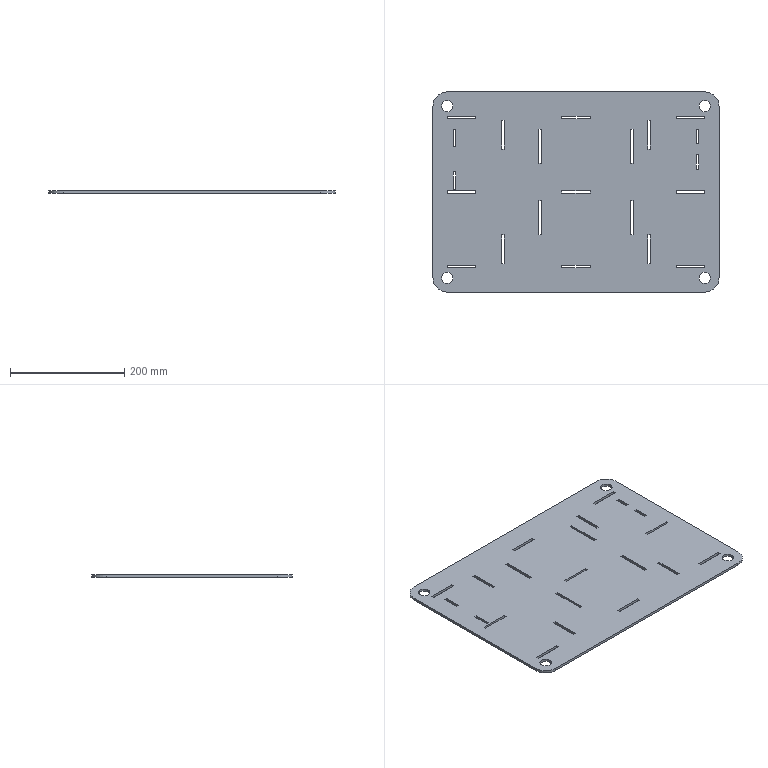Part | SolidWorks | features FlatPattern 1, SMBaseFlange 1, SheetMetal 1 | 1 solid | 102 faces | box 500 x 350 x 4.5 mm | volume 759181 mm3 | plane 90 | cylinder 12 | commonest cylinder face diameters 20 x8 50 x4